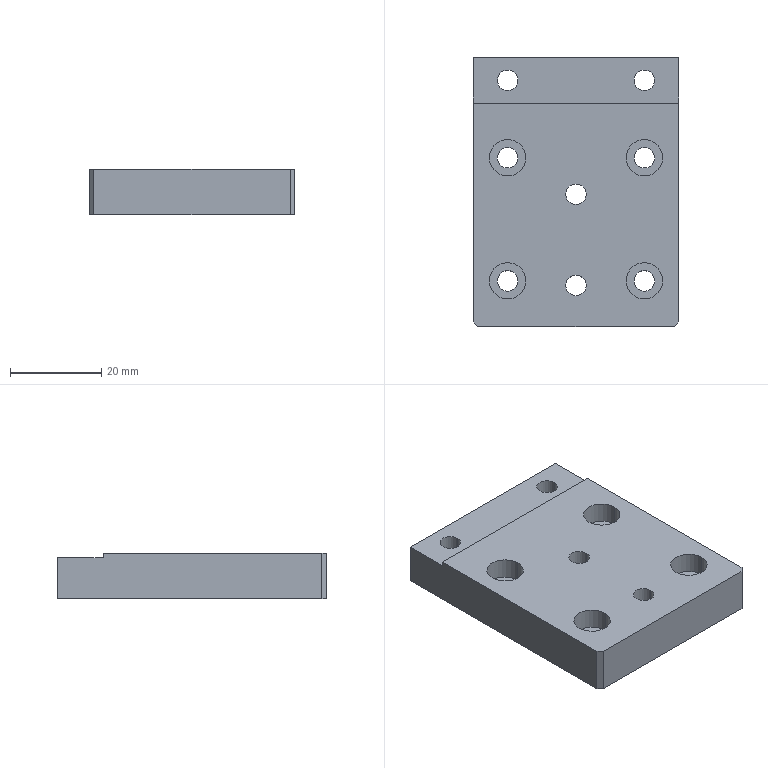Part | STEP file | 2083 Bag feed connecting plate B | 1 solid | 50 faces | box 45 x 59 x 10 mm | volume 23585 mm3 | cylinder 32 | plane 18 | commonest cylinder face diameters 4.5 x16 8 x16